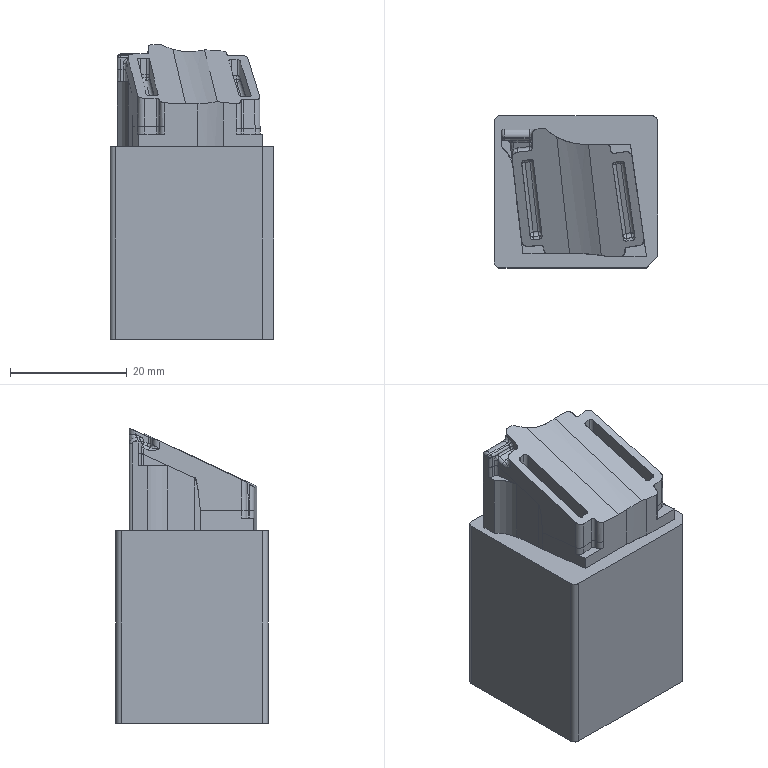NC program | NX | posted with a generic post | part box 28 x 26 x 50.455 mm
Whole program:
N10 G17 G21 G94 G90
(CAVITY_MILL_COPY_COPY , TOOL : MILL_2)
N12 T00 M6
N14 G54
N16 G17 G0 G90 X-14.496 Y12.325 S0 M3
N18 G43 Z10. H0
N20 Z-0.037
N22 G94 G1 Z-0.337 F250.
N24 X-13.997
N26 G3 X-10.997 Y9.325 R3.
N28 G1 X-9.23
N30 G2 X-8.224 Y10.006 R1.
N32 G1 Y9.972
N34 X-8.238 Y9.844
N36 G3 X-8.224 Y9.604 R0.772
N38 G1 X-8.223 Y9.02
N40 Y9.016
N42 X-8.193 Y8.822
N44 X-8.192 Y8.813
N46 X-8.193 Y8.451
N48 X-8.176 Y8.175
N50 Y8.168
N52 X-8.193 Y7.889
N54 Y7.705
N56 X-8.175 Y7.66
N58 X-8.223 Y7.653
N60 X-8.222 Y6.701
N62 X-8.235 Y6.699
N64 X-8.509 Y6.67
N66 X-8.781 Y6.639
N68 X-8.835 Y6.632
N70 X-8.877 Y6.628
N72 X-8.919 Y6.622
N74 X-8.93 Y6.621
N76 X-8.962 Y6.616
N78 X-9.071 Y6.605
N80 X-9.078 Y6.604
N82 X-9.335 Y6.574
N84 X-9.34 Y6.573
N86 X-9.475 Y6.558
N88 X-9.537 Y6.55
N90 X-9.569 Y6.546
N92 X-9.688 Y6.538
N94 X-9.815 Y6.524
N96 X-9.884 Y6.511
N98 X-10.081 Y6.481
N100 X-10.09 Y6.478
N102 G2 X-10.266 Y6.367 R1.
N104 G1 X-10.453 Y6.274
N106 X-10.499 Y6.228
N108 X-10.528 Y6.189
N110 X-10.552 Y6.155
N112 X-10.588 Y6.093
N114 X-10.592 Y6.085
N116 X-10.651 Y5.932
N118 X-10.661 Y5.89
N120 X-10.673 Y5.816
N122 Y5.536
N124 G2 X-12.665 Y5.416 R1.
N126 X-12.582 Y6.741 R3.632
N128 G1 X-12.559 Y6.816
N130 X-12.496 Y7.003
N132 G2 X-13.262 Y7.975 R1.
N134 G1 X-13.263 Y8.325
N136 G2 X-12.263 Y9.325 R1.
N138 G1 X-10.997
N140 Y9.075
N142 X-9.23
N144 G3 X-8.993 Y9.246 R0.25
N146 G2 X-8.491 Y9.728 R0.75
N148 G1 X-8.474 Y9.579
N150 X-8.473 Y8.993
N152 X-8.469 Y8.972
N154 X-8.442 Y8.799
N156 X-8.443 Y8.444
N158 X-8.427 Y8.171
N160 X-8.443 Y7.897
N162 Y7.772
N164 X-8.495 Y7.722
N166 X-8.473 Y7.653
N168 Y6.925
N170 X-8.536 Y6.918
N172 X-8.81 Y6.887
N174 X-8.865 Y6.88
N176 X-8.896 Y6.877
N178 X-8.906
N180 X-8.916 Y6.875
N182 X-8.948 Y6.871
N184 X-8.963 Y6.869
N186 X-9.001 Y6.863
N188 X-9.092 Y6.854
N190 X-9.102 Y6.853
N192 X-9.601 Y6.794
N194 X-9.703 Y6.788
N196 X-9.856 Y6.771
N198 X-9.869 Y6.768
N200 X-9.921 Y6.758
N202 X-10.136 Y6.725
N204 X-10.207 Y6.734
N206 X-10.245 Y6.674
N208 X-10.377 Y6.591
N210 X-10.564 Y6.498
N212 X-10.629 Y6.451
N214 X-10.688 Y6.393
N216 X-10.731 Y6.336
N218 X-10.763 Y6.29
N220 X-10.807 Y6.214
N222 X-10.821 Y6.188
N224 X-10.891 Y6.005
N226 X-10.906 Y5.937
N228 X-10.923 Y5.836
N230 Y5.536
N232 G2 X-12.417 Y5.446 R0.75
N234 X-12.322 Y6.736 R3.382
N236 G1 X-12.259 Y6.923
N238 G3 X-12.438 Y7.246 R0.25
N240 G2 X-13.012 Y7.975 R0.75
N242 G1 X-13.013 Y8.325
N244 G2 X-12.263 Y9.075 R0.75
N246 G1 X-10.997
N248 Y8.825
N250 X-9.23
N252 G3 X-8.756 Y9.166 R0.5
N254 G1 X-8.724 Y9.242
N256 X-8.723 Y8.965
N258 X-8.715 Y8.926
N260 X-8.692 Y8.78
N262 X-8.693 Y8.437
N264 X-8.677 Y8.172
N266 X-8.693 Y7.904
N268 Y7.824
N270 X-8.745 Y7.745
N272 X-8.723 Y7.652
N274 Y7.149
N276 X-8.839 Y7.135
N278 X-8.891 Y7.129
N280 X-8.918 Y7.126
N282 X-8.935 Y7.125
N284 X-8.953 Y7.122
N286 X-8.979 Y7.119
N288 X-8.997 Y7.117
N290 X-9.041 Y7.11
N292 X-9.113 Y7.104
N294 X-9.132 Y7.101
N296 X-9.631 Y7.042
N298 X-9.716 Y7.039
N300 X-9.898 Y7.017
N302 X-9.92 Y7.013
N304 X-9.963 Y7.004
N306 X-10.179 Y6.972
N308 G3 X-10.401 Y6.87 R0.5
N310 G1 X-10.489 Y6.815
N312 X-10.675 Y6.722
N314 X-10.806 Y6.629
N316 X-10.878 Y6.557
N318 X-10.933 Y6.482
N320 X-10.974 Y6.425
N322 X-11.026 Y6.335
N324 X-11.049 Y6.291
N326 X-11.131 Y6.077
N328 X-11.152 Y5.984
N330 X-11.173 Y5.856
N332 Y5.536
N334 G2 X-12.169 Y5.476 R0.5
N336 X-12.083 Y6.663 R3.132
N338 G1 X-12.022 Y6.843
N340 G3 X-12.379 Y7.489 R0.5
N342 G2 X-12.762 Y7.975 R0.5
N344 G1 X-12.763 Y8.325
N346 G2 X-12.263 Y8.825 R0.5
N348 G1 X-10.997
N350 Y8.575
N352 X-9.23
N354 G3 X-8.942 Y8.633 R0.75
N356 G1 X-8.943 Y8.43
N358 X-8.928 Y8.172
N360 X-8.943 Y7.912
N362 Y7.864
N364 G3 X-8.973 Y7.652 R0.75
N366 G1 Y7.372
N368 X-8.989 Y7.37
N370 X-9.01 Y7.367
N372 X-9.031 Y7.364
N374 X-9.08 Y7.357
N376 X-9.13 Y7.353
N378 X-9.162 Y7.349
N380 X-9.662 Y7.291
N382 X-9.726 Y7.289
N384 X-9.94 Y7.264
N386 X-9.97 Y7.258
N388 X-10.005 Y7.251
N390 X-10.221 Y7.218
N392 G3 X-10.557 Y7.065 R0.75
N394 G1 X-10.6 Y7.039
N396 X-10.786 Y6.946
N398 G3 X-10.982 Y6.806 R0.75
N400 G1 X-11.067 Y6.721
N402 X-11.136 Y6.629
N404 X-11.184 Y6.56
N406 X-11.245 Y6.455
N408 X-11.277 Y6.393
N410 X-11.371 Y6.15
N412 X-11.398 Y6.031
N414 X-11.423 Y5.876
N416 Y5.536
N418 G2 X-11.921 Y5.506 R0.25
N420 X-11.844 Y6.591 R2.882
N422 G1 X-11.786 Y6.763
N424 G3 X-12.321 Y7.732 R0.75
N426 G2 X-12.512 Y7.975 R0.25
N428 G1 X-12.513 Y8.325
N430 G2 X-12.263 Y8.575 R0.25
N432 G1 X-10.997
N434 X-10.996 Y8.325
N436 X-9.187 Y8.326
N438 X-9.178 Y8.172
N440 X-9.193 Y7.919
N442 Y7.897
N444 G3 X-9.223 Y7.652 R1.
N446 G1 Y7.594
N448 X-9.695 Y7.538
N450 X-9.7
N452 X-9.727 Y7.541
N454 X-9.982 Y7.511
N456 X-10.02 Y7.502
N458 X-10.046 Y7.498
N460 X-10.262 Y7.465
N462 G3 X-10.711 Y7.263 R1.
N464 G1 X-10.897 Y7.17
N466 G3 X-11.158 Y6.983 R1.
N468 G1 X-11.257 Y6.885
N470 X-11.339 Y6.775
N472 X-11.395 Y6.695
N474 X-11.464 Y6.576
N476 X-11.506 Y6.496
N478 X-11.611 Y6.223
N480 X-11.643 Y6.079
N482 X-11.673 Y5.896
N484 Y5.536
N486 G2 X-11.604 Y6.519 R2.632
N488 G1 X-11.549 Y6.683
N490 G3 X-12.262 Y7.975 R1.
N492 G1 X-12.263 Y8.325
N494 X-10.996
N496 Y8.075
N498 X-9.434 Y8.076
N500 X-9.443 Y7.926
N502 X-9.463 Y7.817
N504 X-9.702 Y7.789
N506 X-9.729 Y7.792
N508 X-10.024 Y7.758
N510 X-10.071 Y7.747
N512 X-10.088 Y7.744
N514 X-10.302 Y7.712
N516 G3 X-10.844 Y7.475 R1.25
N518 G1 X-11.008 Y7.394
N520 G3 X-11.266 Y7.224 R1.25
N522 X-11.853 Y8.075 R1.25
N524 G1 X-10.996
N526 Y7.825
N528 X-10.751 Y7.826
N530 G3 X-10.976 Y7.689 R1.5
N532 G1 X-11.119 Y7.618
N534 X-11.126 Y7.615
N536 G3 X-11.242 Y7.825 R1.5
N538 G1 X-10.996
N540 G3 X-9.497 Y9.326 R1.5
N542 G1 Z-0.037
N544 G0 Z0.3
N546 X-14.496 Y12.325
N548 Z-0.374
N550 G1 Z-0.674
N552 X-13.997
N554 G3 X-10.997 Y9.325 R3.
N556 G1 X-9.23
N558 G2 X-8.228 Y10.006 R1.
N560 G3 X-8.252 Y9.716 R1.75
N562 G1 Y9.152
N564 G3 X-8.192 Y8.769 R0.811
N566 G1 X-8.193 Y8.451
N568 X-8.176 Y8.175
N570 Y8.168
N572 X-8.193 Y7.889
N574 Y7.705
N576 X-8.175 Y7.66
N578 X-8.223 Y7.653
N580 X-8.222 Y6.701
N582 X-8.235 Y6.699
N584 X-8.509 Y6.67
N586 X-8.781 Y6.639
N588 X-8.835 Y6.632
N590 X-8.877 Y6.628
N592 X-8.919 Y6.622
N594 X-8.93 Y6.621
N596 X-8.962 Y6.616
N598 X-9.071 Y6.605
N600 X-9.078 Y6.604
N602 X-9.335 Y6.574
N604 X-9.34 Y6.573
N606 X-9.475 Y6.558
N608 X-9.537 Y6.55
N610 X-9.569 Y6.546
N612 X-9.688 Y6.538
N614 X-9.815 Y6.524
N616 X-9.884 Y6.511
N618 X-10.081 Y6.481
N620 X-10.09 Y6.478
N622 G2 X-10.266 Y6.367 R1.
N624 G1 X-10.453 Y6.274
N626 X-10.499 Y6.228
N628 X-10.528 Y6.189
N630 X-10.552 Y6.155
N632 X-10.588 Y6.093
N634 X-10.592 Y6.085
N636 X-10.651 Y5.932
N638 X-10.661 Y5.89
N640 X-10.673 Y5.816
N642 Y5.536
N644 G2 X-12.665 Y5.416 R1.
N646 X-12.582 Y6.741 R3.632
N648 G1 X-12.559 Y6.816
N650 X-12.496 Y7.003
N652 G2 X-13.262 Y7.975 R1.
N654 G1 X-13.263 Y8.325
N656 G2 X-12.263 Y9.325 R1.
N658 G1 X-10.997
N660 Y9.075
N662 X-9.23
N664 G3 X-8.993 Y9.246 R0.25
N666 G2 X-8.502 Y9.724 R0.75
N668 G1 Y9.715
N670 Y9.162
N672 G3 X-8.442 Y8.722 R1.061
N674 G1 X-8.443 Y8.444
N676 X-8.427 Y8.171
N678 X-8.443 Y7.897
N680 Y7.772
N682 X-8.495 Y7.722
N684 X-8.473 Y7.653
N686 Y6.925
N688 X-8.536 Y6.918
N690 X-8.81 Y6.887
N692 X-8.865 Y6.88
N694 X-8.896 Y6.877
N696 X-8.906
N698 X-8.916 Y6.875
N700 X-9.001 Y6.863
N702 X-9.092 Y6.854
N704 X-9.102 Y6.853
N706 X-9.108 Y6.852
N708 X-9.364 Y6.822
N710 X-9.368 Y6.821
N712 X-9.504 Y6.806
N714 X-9.568 Y6.798
N716 X-9.703 Y6.788
N718 X-9.856 Y6.771
N720 X-9.869 Y6.768
N722 X-9.921 Y6.758
N724 X-10.136 Y6.725
N726 X-10.207 Y6.734
N728 X-10.245 Y6.674
N730 X-10.377 Y6.591
N732 X-10.564 Y6.498
N734 X-10.629 Y6.451
N736 X-10.688 Y6.393
N738 X-10.731 Y6.336
N740 X-10.763 Y6.29
N742 X-10.807 Y6.214
N744 X-10.821 Y6.188
N746 X-10.891 Y6.005
N748 X-10.906 Y5.937
N750 X-10.923 Y5.836
N752 Y5.536
N754 G2 X-12.417 Y5.446 R0.75
N756 X-12.322 Y6.736 R3.382
N758 G1 X-12.259 Y6.923
N760 G3 X-12.438 Y7.246 R0.25
N762 G2 X-13.012 Y7.975 R0.75
N764 G1 X-13.013 Y8.325
N766 G2 X-12.263 Y9.075 R0.75
N768 G1 X-10.997
N770 Y8.825
N772 X-9.23
N774 G3 X-8.756 Y9.166 R0.5
N776 G1 X-8.752 Y9.178
N778 G3 X-8.692 Y8.681 R1.311
N780 G1 X-8.693 Y8.437
N782 X-8.677 Y8.172
N784 X-8.693 Y7.904
N786 Y7.824
N788 X-8.745 Y7.745
N790 X-8.723 Y7.652
N792 Y7.149
N794 X-8.839 Y7.135
N796 X-8.891 Y7.129
N798 X-8.918 Y7.126
N800 X-8.935 Y7.125
N802 X-8.954 Y7.122
N804 X-9.039 Y7.11
N806 X-9.113 Y7.104
N808 X-9.133 Y7.101
N810 X-9.137 Y7.1
N812 X-9.393 Y7.07
N814 X-9.396
N816 X-9.533 Y7.055
N818 X-9.603 Y7.046
N820 X-9.715 Y7.039
N822 X-9.898 Y7.017
N824 X-9.92 Y7.013
N826 X-9.963 Y7.004
N828 X-10.179 Y6.972
N830 G3 X-10.401 Y6.87 R0.5
N832 G1 X-10.489 Y6.815
N834 X-10.675 Y6.722
N836 X-10.806 Y6.629
N838 X-10.878 Y6.557
N840 X-10.933 Y6.482
N842 X-10.974 Y6.425
N844 X-11.026 Y6.335
N846 X-11.049 Y6.291
N848 X-11.131 Y6.077
N850 X-11.152 Y5.984
N852 X-11.173 Y5.856
N854 Y5.536
N856 G2 X-12.169 Y5.476 R0.5
N858 X-12.083 Y6.663 R3.132
N860 G1 X-12.022 Y6.843
N862 G3 X-12.379 Y7.489 R0.5
N864 G2 X-12.762 Y7.975 R0.5
N866 G1 X-12.763 Y8.325
N868 G2 X-12.263 Y8.825 R0.5
N870 G1 X-10.997
N872 Y8.575
N874 X-9.23
N876 G3 X-8.942 Y8.633 R0.75
N878 G1 X-8.943 Y8.43
N880 X-8.928 Y8.172
N882 X-8.943 Y7.912
N884 Y7.864
N886 G3 X-8.973 Y7.652 R0.75
N888 G1 Y7.372
N890 X-8.991 Y7.37
N892 X-9.077 Y7.357
N894 X-9.13 Y7.353
N896 X-9.163 Y7.349
N898 X-9.167
N900 X-9.422 Y7.319
N902 X-9.425 Y7.318
N904 X-9.562 Y7.303
N906 X-9.641 Y7.293
N908 X-9.724 Y7.289
N910 X-9.94 Y7.264
N912 X-9.97 Y7.258
N914 X-10.005 Y7.251
N916 X-10.221 Y7.218
N918 G3 X-10.557 Y7.065 R0.75
N920 G1 X-10.6 Y7.039
N922 X-10.786 Y6.946
N924 G3 X-10.982 Y6.806 R0.75
N926 G1 X-11.067 Y6.721
N928 X-11.136 Y6.629
N930 X-11.184 Y6.56
N932 X-11.245 Y6.455
N934 X-11.277 Y6.393
N936 X-11.371 Y6.15
N938 X-11.398 Y6.031
N940 X-11.423 Y5.876
N942 Y5.536
N944 G2 X-11.921 Y5.506 R0.25
N946 X-11.844 Y6.591 R2.882
N948 G1 X-11.786 Y6.763
N950 G3 X-12.321 Y7.732 R0.75
N952 G2 X-12.512 Y7.975 R0.25
N954 G1 X-12.513 Y8.325
N956 G2 X-12.263 Y8.575 R0.25
N958 G1 X-10.997
N960 X-10.996 Y8.325
N962 X-9.187 Y8.326
N964 X-9.178 Y8.172
N966 X-9.193 Y7.919
N968 Y7.897
N970 G3 X-9.223 Y7.652 R1.
N972 G1 Y7.594
N974 X-9.451 Y7.567
N976 X-9.453
N978 X-9.591 Y7.551
N980 X-9.683 Y7.54
N982 X-9.694 Y7.537
N984 X-9.724 Y7.541
N986 X-9.982 Y7.511
N988 X-10.02 Y7.502
N990 X-10.046 Y7.498
N992 X-10.262 Y7.465
N994 G3 X-10.711 Y7.263 R1.
N996 G1 X-10.897 Y7.17
N998 G3 X-11.158 Y6.983 R1.
N1000 G1 X-11.257 Y6.885
N1002 X-11.339 Y6.775
N1004 X-11.395 Y6.695
N1006 X-11.464 Y6.576
N1008 X-11.506 Y6.496
N1010 X-11.611 Y6.223
N1012 X-11.643 Y6.079
N1014 X-11.673 Y5.896
N1016 Y5.536
N1018 G2 X-11.604 Y6.519 R2.632
N1020 G1 X-11.549 Y6.683
N1022 G3 X-12.262 Y7.975 R1.
N1024 G1 X-12.263 Y8.325
N1026 X-10.996
N1028 Y8.075
N1030 X-9.434 Y8.076
N1032 X-9.443 Y7.926
N1034 X-9.463 Y7.817
N1036 X-9.48 Y7.815
N1038 X-9.481
N1040 X-9.62 Y7.799
N1042 X-9.699 Y7.79
N1044 X-9.723 Y7.793
N1046 X-10.024 Y7.758
N1048 X-10.071 Y7.747
N1050 X-10.088 Y7.744
N1052 X-10.302 Y7.712
N1054 G3 X-10.844 Y7.475 R1.25
N1056 G1 X-11.008 Y7.394
N1058 G3 X-11.266 Y7.224 R1.25
N1060 X-11.853 Y8.075 R1.25
N1062 G1 X-10.996
N1064 Y7.825
N1066 X-10.751 Y7.826
N1068 G3 X-10.976 Y7.689 R1.5
N1070 G1 X-11.119 Y7.618
N1072 X-11.126 Y7.615
N1074 G3 X-11.242 Y7.825 R1.5
N1076 G1 X-10.996
N1078 G3 X-9.497 Y9.326 R1.5
N1080 G1 Z-0.374
N1082 G0 Z0.3
N1084 X-14.496 Y12.325
N1086 Z-0.71
N1088 G1 Z-1.01
N1090 X-13.997
N1092 G3 X-10.997 Y9.325 R3.
N1094 G1 X-9.23
N1096 G2 X-8.234 Y10.006 R1.
N1098 G3 X-8.254 Y9.612 R1.746
N1100 G1 X-8.253 Y8.425
N1102 G3 X-8.185 Y8.024 R0.811
N1104 G1 X-8.193 Y7.889
N1106 Y7.705
N1108 X-8.175 Y7.66
N1110 X-8.223 Y7.653
N1112 X-8.222 Y6.701
N1114 X-8.235 Y6.699
N1116 X-8.509 Y6.67
N1118 X-8.781 Y6.639
N1120 X-8.835 Y6.632
N1122 X-8.877 Y6.628
N1124 X-8.919 Y6.622
N1126 X-8.93 Y6.621
N1128 X-8.962 Y6.616
N1130 X-9.071 Y6.605
N1132 X-9.078 Y6.604
N1134 X-9.335 Y6.574
N1136 X-9.34 Y6.573
N1138 X-9.475 Y6.558
N1140 X-9.537 Y6.55
N1142 X-9.569 Y6.546
N1144 X-9.688 Y6.538
N1146 X-9.815 Y6.524
N1148 X-9.884 Y6.511
N1150 X-10.081 Y6.481
N1152 X-10.09 Y6.478
N1154 G2 X-10.266 Y6.367 R1.
N1156 G1 X-10.453 Y6.274
N1158 X-10.499 Y6.228
N1160 X-10.528 Y6.189
N1162 X-10.552 Y6.155
N1164 X-10.588 Y6.093
N1166 X-10.592 Y6.085
N1168 X-10.651 Y5.932
N1170 X-10.661 Y5.89
N1172 X-10.673 Y5.816
N1174 Y5.536
N1176 G2 X-12.665 Y5.416 R1.
N1178 X-12.582 Y6.741 R3.632
N1180 G1 X-12.559 Y6.816
N1182 X-12.496 Y7.003
N1184 G2 X-13.262 Y7.975 R1.
N1186 G1 X-13.263 Y8.325
N1188 G2 X-12.263 Y9.325 R1.
N1190 G1 X-10.997
N1192 Y9.075
N1194 X-9.23
N1196 G3 X-8.993 Y9.246 R0.25
N1198 G2 X-8.507 Y9.723 R0.75
N1200 G1 X-8.504 Y9.604
N1202 X-8.503 Y8.435
N1204 G3 X-8.438 Y7.982 R1.061
N1206 G1 X-8.443 Y7.897
N1208 Y7.772
N1210 X-8.495 Y7.722
N1212 X-8.473 Y7.653
N1214 Y6.925
N1216 X-8.536 Y6.918
N1218 X-8.81 Y6.887
N1220 X-8.865 Y6.88
N1222 X-8.896 Y6.877
N1224 X-8.906
N1226 X-8.916 Y6.875
N1228 X-9.001 Y6.863
N1230 X-9.092 Y6.854
N1232 X-9.102 Y6.853
N1234 X-9.108 Y6.852
N1236 X-9.364 Y6.822
N1238 X-9.601 Y6.794
N1240 X-9.703 Y6.788
N1242 X-9.856 Y6.771
N1244 X-9.869 Y6.768
N1246 X-9.921 Y6.758
N1248 X-10.136 Y6.725
N1250 X-10.207 Y6.734
N1252 X-10.245 Y6.674
N1254 X-10.377 Y6.591
N1256 X-10.564 Y6.498
N1258 X-10.629 Y6.451
N1260 X-10.688 Y6.393
N1262 X-10.731 Y6.336
N1264 X-10.763 Y6.29
N1266 X-10.807 Y6.214
N1268 X-10.821 Y6.188
N1270 X-10.891 Y6.005
N1272 X-10.906 Y5.937
N1274 X-10.923 Y5.836
N1276 Y5.536
N1278 G2 X-12.417 Y5.446 R0.75
N1280 X-12.322 Y6.736 R3.382
N1282 G1 X-12.259 Y6.923
N1284 G3 X-12.438 Y7.246 R0.25
N1286 G2 X-13.012 Y7.975 R0.75
N1288 G1 X-13.013 Y8.325
N1290 G2 X-12.263 Y9.075 R0.75
N1292 G1 X-10.997
N1294 Y8.825
N1296 X-9.23
N1298 G3 X-8.756 Y9.166 R0.5
N1300 G1 X-8.753 Y9.173
N1302 Y8.444
N1304 G3 X-8.691 Y7.947 R1.311
N1306 G1 X-8.693 Y7.904
N1308 Y7.824
N1310 X-8.745 Y7.745
N1312 X-8.723 Y7.652
N1314 Y7.149
N1316 X-8.839 Y7.135
N1318 X-8.891 Y7.129
N1320 X-8.918 Y7.126
N1322 X-8.935 Y7.125
N1324 X-8.954 Y7.122
N1326 X-9.039 Y7.11
N1328 X-9.113 Y7.104
N1330 X-9.133 Y7.101
N1332 X-9.137 Y7.1
N1334 X-9.393 Y7.07
N1336 X-9.631 Y7.042
N1338 X-9.716 Y7.039
N1340 X-9.898 Y7.017
N1342 X-9.92 Y7.013
N1344 X-9.963 Y7.004
N1346 X-10.179 Y6.972
N1348 G3 X-10.401 Y6.87 R0.5
N1350 G1 X-10.489 Y6.815
N1352 X-10.675 Y6.722
N1354 X-10.806 Y6.629
N1356 X-10.878 Y6.557
N1358 X-10.933 Y6.482
N1360 X-10.974 Y6.425
N1362 X-11.026 Y6.335
N1364 X-11.049 Y6.291
N1366 X-11.131 Y6.077
N1368 X-11.152 Y5.984
N1370 X-11.173 Y5.856
N1372 Y5.536
N1374 G2 X-12.169 Y5.476 R0.5
N1376 X-12.083 Y6.663 R3.132
N1378 G1 X-12.022 Y6.843
N1380 G3 X-12.379 Y7.489 R0.5
N1382 G2 X-12.762 Y7.975 R0.5
N1384 G1 X-12.763 Y8.325
N1386 G2 X-12.263 Y8.825 R0.5
N1388 G1 X-10.997
N1390 Y8.575
N1392 X-9.23
N1394 G3 X-9.003 Y8.611 R0.75
N1396 G1 Y8.452
N1398 G3 X-8.943 Y7.912 R1.561
N1400 G1 Y7.864
N1402 G3 X-8.973 Y7.652 R0.75
N1404 G1 Y7.372
N1406 X-8.991 Y7.37
N1408 X-9.077 Y7.357
N1410 X-9.13 Y7.353
N1412 X-9.163 Y7.349
N1414 X-9.167
N1416 X-9.423 Y7.319
N1418 X-9.662 Y7.291
N1420 X-9.726 Y7.289
N1422 X-9.94 Y7.264
N1424 X-9.97 Y7.258
N1426 X-10.005 Y7.251
N1428 X-10.221 Y7.218
N1430 G3 X-10.557 Y7.065 R0.75
N1432 G1 X-10.6 Y7.039
N1434 X-10.786 Y6.946
N1436 G3 X-10.982 Y6.806 R0.75
N1438 G1 X-11.067 Y6.721
N1440 X-11.136 Y6.629
N1442 X-11.184 Y6.56
N1444 X-11.245 Y6.455
N1446 X-11.277 Y6.393
N1448 X-11.371 Y6.15
N1450 X-11.398 Y6.031
N1452 X-11.423 Y5.876
N1454 Y5.536
N1456 G2 X-11.921 Y5.506 R0.25
N1458 X-11.844 Y6.591 R2.882
N1460 G1 X-11.786 Y6.763
N1462 G3 X-12.321 Y7.732 R0.75
N1464 G2 X-12.512 Y7.975 R0.25
N1466 G1 X-12.513 Y8.325
N1468 G2 X-12.263 Y8.575 R0.25
N1470 G1 X-10.997
N1472 X-10.996 Y8.325
N1474 X-9.256
N1476 G3 X-9.196 Y7.886 R1.811
N1478 X-9.223 Y7.652 R1.
N1480 G1 Y7.594
N1482 X-9.452 Y7.567
N1484 X-9.695 Y7.538
N1486 X-9.7
N1488 X-9.727 Y7.541
N1490 X-9.982 Y7.511
N1492 X-10.02 Y7.502
N1494 X-10.046 Y7.498
N1496 X-10.262 Y7.465
N1498 G3 X-10.711 Y7.263 R1.
N1500 G1 X-10.897 Y7.17
N1502 G3 X-11.158 Y6.983 R1.
N1504 G1 X-11.257 Y6.885
N1506 X-11.339 Y6.775
N1508 X-11.395 Y6.695
N1510 X-11.464 Y6.576
N1512 X-11.506 Y6.496
N1514 X-11.611 Y6.223
N1516 X-11.643 Y6.079
N1518 X-11.673 Y5.896
N1520 Y5.536
N1522 G2 X-11.604 Y6.519 R2.632
N1524 G1 X-11.549 Y6.683
N1526 G3 X-12.262 Y7.975 R1.
N1528 G1 X-12.263 Y8.325
N1530 X-10.996
N1532 Y8.075
N1534 X-9.488
N1536 X-9.452 Y7.882
N1538 X-9.463 Y7.817
N1540 X-9.481 Y7.815
N1542 X-9.702 Y7.789
N1544 X-9.728 Y7.792
N1546 X-10.024 Y7.758
N1548 X-10.071 Y7.747
N1550 X-10.088 Y7.744
N1552 X-10.302 Y7.712
N1554 G3 X-10.844 Y7.475 R1.25
N1556 G1 X-11.008 Y7.394
N1558 G3 X-11.266 Y7.224 R1.25
N1560 X-11.853 Y8.075 R1.25
N1562 G1 X-10.996
N1564 Y7.825
N1566 X-10.752
N1568 G3 X-10.976 Y7.689 R1.5
N1570 G1 X-11.119 Y7.618
N1572 X-11.126 Y7.615
N1574 G3 X-11.241 Y7.825 R1.5
N1576 G1 X-10.996
N1578 G3 X-9.497 Y9.325 R1.5
N1580 G1 Z-0.71
N1582 G0 Z0.3
N1584 X-14.496 Y12.325
N1586 Z-1.047
N1588 G1 Z-1.347
N1590 X-13.997
N1592 G3 X-10.997 Y9.325 R3.
N1594 G1 X-9.23
N1596 G2 X-8.344 Y10.005 R1.
N1598 G3 X-8.264 Y9.007 R1.821
N1600 G1 X-8.255 Y8.898
N1602 X-8.253 Y7.698
N1604 G3 X-8.223 Y7.397 R0.811
N1606 G1 X-8.222 Y6.701
N1608 X-8.235 Y6.699
N1610 X-8.509 Y6.67
N1612 X-8.781 Y6.639
N1614 X-8.835 Y6.632
N1616 X-8.877 Y6.628
N1618 X-8.919 Y6.622
N1620 X-8.93 Y6.621
N1622 X-8.962 Y6.616
N1624 X-9.071 Y6.605
N1626 X-9.078 Y6.604
N1628 X-9.335 Y6.574
N1630 X-9.34 Y6.573
N1632 X-9.475 Y6.558
N1634 X-9.537 Y6.55
N1636 X-9.569 Y6.546
N1638 X-9.688 Y6.538
N1640 X-9.815 Y6.524
N1642 X-9.884 Y6.511
N1644 X-10.081 Y6.481
N1646 X-10.09 Y6.478
N1648 G2 X-10.266 Y6.367 R1.
N1650 G1 X-10.453 Y6.274
N1652 X-10.499 Y6.228
N1654 X-10.528 Y6.189
N1656 X-10.552 Y6.155
N1658 X-10.588 Y6.093
N1660 X-10.592 Y6.085
N1662 X-10.651 Y5.932
N1664 X-10.661 Y5.89
N1666 X-10.673 Y5.816
N1668 Y5.536
N1670 G2 X-12.665 Y5.416 R1.
N1672 X-12.582 Y6.741 R3.632
N1674 G1 X-12.559 Y6.816
N1676 X-12.496 Y7.003
N1678 G2 X-13.262 Y7.975 R1.
N1680 G1 X-13.263 Y8.325
N1682 G2 X-12.263 Y9.325 R1.
N1684 G1 X-10.997
N1686 Y9.075
N1688 X-9.23
N1690 G3 X-8.993 Y9.246 R0.25
N1692 G2 X-8.63 Y9.672 R0.75
N1694 G3 X-8.511 Y8.953 R2.071
N1696 G1 X-8.505 Y8.887
N1698 X-8.504 Y7.708
N1700 G3 X-8.473 Y7.363 R1.061
N1702 G1 Y6.925
N1704 X-8.536 Y6.918
N1706 X-8.81 Y6.887
N1708 X-8.865 Y6.88
N1710 X-8.896 Y6.877
N1712 X-8.906
N1714 X-8.916 Y6.875
N1716 X-8.948 Y6.871
N1718 X-8.963 Y6.869
N1720 X-9.001 Y6.863
N1722 X-9.092 Y6.854
N1724 X-9.102 Y6.853
N1726 X-9.108 Y6.852
N1728 X-9.364 Y6.822
N1730 X-9.601 Y6.794
N1732 X-9.703 Y6.788
N1734 X-9.856 Y6.771
N1736 X-9.869 Y6.768
N1738 X-9.921 Y6.758
N1740 X-10.136 Y6.725
N1742 X-10.207 Y6.734
N1744 X-10.245 Y6.674
N1746 X-10.377 Y6.591
N1748 X-10.564 Y6.498
N1750 X-10.629 Y6.451
N1752 X-10.688 Y6.393
N1754 X-10.731 Y6.336
N1756 X-10.763 Y6.29
N1758 X-10.807 Y6.214
N1760 X-10.821 Y6.188
N1762 X-10.891 Y6.005
N1764 X-10.906 Y5.937
N1766 X-10.923 Y5.836
N1768 Y5.536
N1770 G2 X-12.417 Y5.446 R0.75
N1772 X-12.322 Y6.736 R3.382
N1774 G1 X-12.259 Y6.923
N1776 G3 X-12.438 Y7.246 R0.25
N1778 G2 X-13.012 Y7.975 R0.75
N1780 G1 X-13.013 Y8.325
N1782 G2 X-12.263 Y9.075 R0.75
N1784 G1 X-10.997
N1786 Y8.825
N1788 X-9.23
N1790 G3 X-8.805 Y9.061 R0.5
N1792 G1 X-8.757 Y8.9
N1794 X-8.755 Y8.876
N1796 X-8.754 Y7.717
N1798 G3 X-8.723 Y7.333 R1.311
N1800 G1 Y7.149
N1802 X-8.839 Y7.135
N1804 X-8.891 Y7.129
N1806 X-8.918 Y7.126
N1808 X-8.935 Y7.125
N1810 X-8.953 Y7.122
N1812 X-8.979 Y7.119
N1814 X-8.997 Y7.117
N1816 X-9.041 Y7.11
N1818 X-9.113 Y7.104
N1820 X-9.133 Y7.101
N1822 X-9.137 Y7.1
N1824 X-9.393 Y7.07
N1826 X-9.631 Y7.042
N1828 X-9.716 Y7.039
N1830 X-9.898 Y7.017
N1832 X-9.92 Y7.013
N1834 X-9.963 Y7.004
N1836 X-10.179 Y6.972
N1838 G3 X-10.401 Y6.87 R0.5
N1840 G1 X-10.489 Y6.815
N1842 X-10.675 Y6.722
N1844 X-10.806 Y6.629
N1846 X-10.878 Y6.557
N1848 X-10.933 Y6.482
N1850 X-10.974 Y6.425
N1852 X-11.026 Y6.335
N1854 X-11.049 Y6.291
N1856 X-11.131 Y6.077
N1858 X-11.152 Y5.984
N1860 X-11.173 Y5.856
N1862 Y5.536
N1864 G2 X-12.169 Y5.476 R0.5
N1866 X-12.083 Y6.663 R3.132
N1868 G1 X-12.022 Y6.843
N1870 G3 X-12.379 Y7.489 R0.5
N1872 G2 X-12.762 Y7.975 R0.5
N1874 G1 X-12.763 Y8.325
N1876 G2 X-12.263 Y8.825 R0.5
N1878 G1 X-10.997
N1880 Y8.575
N1882 X-9.23
N1884 G3 X-9.005 Y8.61 R0.75
N1886 G1 X-9.004 Y7.725
N1888 G3 X-8.985 Y7.37 R1.561
N1890 G1 X-8.989
N1892 X-9.01 Y7.367
N1894 X-9.031 Y7.364
N1896 X-9.08 Y7.357
N1898 X-9.13 Y7.353
N1900 X-9.163 Y7.349
N1902 X-9.167
N1904 X-9.423 Y7.319
N1906 X-9.662 Y7.291
N1908 X-9.726 Y7.289
N1910 X-9.94 Y7.264
N1912 X-9.97 Y7.258
N1914 X-10.005 Y7.251
N1916 X-10.221 Y7.218
N1918 G3 X-10.557 Y7.065 R0.75
N1920 G1 X-10.6 Y7.039
N1922 X-10.786 Y6.946
N1924 G3 X-10.982 Y6.806 R0.75
N1926 G1 X-11.067 Y6.721
N1928 X-11.136 Y6.629
N1930 X-11.184 Y6.56
N1932 X-11.245 Y6.455
N1934 X-11.277 Y6.393
N1936 X-11.371 Y6.15
N1938 X-11.398 Y6.031
N1940 X-11.423 Y5.876
N1942 Y5.536
N1944 G2 X-11.921 Y5.506 R0.25
N1946 X-11.844 Y6.591 R2.882
N1948 G1 X-11.786 Y6.763
N1950 G3 X-12.321 Y7.732 R0.75
N1952 G2 X-12.512 Y7.975 R0.25
N1954 G1 X-12.513 Y8.325
N1956 G2 X-12.263 Y8.575 R0.25
N1958 G1 X-10.997
N1960 X-10.996 Y8.325
N1962 X-9.254
N1964 Y7.732
N1966 X-9.256 Y7.59
N1968 X-9.452 Y7.567
N1970 X-9.695 Y7.538
N1972 X-9.7
N1974 X-9.727 Y7.541
N1976 X-9.982 Y7.511
N1978 X-10.02 Y7.502
N1980 X-10.046 Y7.498
N1982 X-10.262 Y7.465
N1984 G3 X-10.711 Y7.263 R1.
N1986 G1 X-10.897 Y7.17
N1988 G3 X-11.158 Y6.983 R1.
N1990 G1 X-11.257 Y6.885
N1992 X-11.339 Y6.775
N1994 X-11.395 Y6.695
N1996 X-11.464 Y6.576
N1998 X-11.506 Y6.496
N2000 X-11.611 Y6.223
N2002 X-11.643 Y6.079
N2004 X-11.673 Y5.896
N2006 Y5.536
N2008 G2 X-11.604 Y6.519 R2.632
N2010 G1 X-11.549 Y6.683
N2012 G3 X-12.262 Y7.975 R1.
N2014 G1 X-12.263 Y8.325
N2016 X-10.996
N2018 Y8.075
N2020 X-9.504
N2022 Y7.812
N2024 X-9.702 Y7.789
N2026 X-9.728 Y7.792
N2028 X-10.024 Y7.758
N2030 X-10.071 Y7.747
N2032 X-10.088 Y7.744
N2034 X-10.302 Y7.712
N2036 G3 X-10.844 Y7.475 R1.25
N2038 G1 X-11.008 Y7.394
N2040 G3 X-11.266 Y7.224 R1.25
N2042 X-11.853 Y8.075 R1.25
N2044 G1 X-10.996
N2046 Y7.825
N2048 X-10.752
N2050 G3 X-10.976 Y7.689 R1.5
N2052 G1 X-11.119 Y7.618
N2054 X-11.126 Y7.615
N2056 G3 X-11.241 Y7.825 R1.5
N2058 G1 X-10.996
N2060 G3 X-9.497 Y9.325 R1.5
N2062 G1 Z-1.047
N2064 G0 Z0.3
N2066 X-14.496 Y8.614
N2068 Z-1.384
N2070 G1 Z-1.684
N2072 G3 X-12.496 Y7.003 R3.
N2074 G2 X-13.262 Y7.975 R1.
N2076 G1 X-13.263 Y8.325
N2078 X-13.257 Y8.429
N2080 X-12.731 Y8.081
N2082 X-12.322 Y8.082
N2084 X-12.323 Y8.325
N2086 X-12.326 Y8.389
N2088 X-12.263 Y8.385
N2090 X-8.342
N2092 X-8.343 Y8.431
N2094 X-8.346 Y8.482
N2096 X-8.268
N2098 X-8.256 Y8.419
N2100 X-8.255 Y7.706
N2102 X-10.116 Y7.49
N2104 X-10.422 Y7.423
N2106 X-10.532 Y7.389
N2108 X-10.541 Y7.383
N2110 X-10.562 Y7.377
N2112 X-10.704 Y7.311
N2114 G3 X-11.267 Y6.775 R1.186
N2116 G1 X-11.274 Y6.761
N2118 X-11.29 Y6.74
N2120 X-11.345 Y6.662
N2122 X-11.412 Y6.547
N2124 X-11.451 Y6.471
N2126 X-11.545 Y6.228
N2128 X-11.555 Y6.2
N2130 X-11.584 Y6.067
N2132 X-11.613 Y5.891
N2134 Y5.536
N2136 X-11.593 Y5.495
N2138 X-11.638 Y5.487
N2140 X-11.528 Y4.547
N2142 G2 X-12.665 Y5.416 R1.
N2144 X-12.582 Y6.741 R3.632
N2146 G1 X-12.559 Y6.816
N2148 X-12.496 Y7.003
N2150 X-12.259 Y6.923
N2152 G3 X-12.438 Y7.246 R0.25
N2154 G2 X-13.012 Y7.968 R0.75
N2156 G1 X-12.869 Y7.873
N2158 X-12.811 Y7.813
N2160 X-12.73 Y7.831
N2162 X-12.322 Y7.832
N2164 G3 X-12.072 Y8.082 R0.25
N2166 G1 Y8.135
N2168 X-8.506
N2170 Y7.929
N2172 X-10.157 Y7.737
N2174 X-10.475 Y7.667
N2176 X-10.494 Y7.662
N2178 X-10.605 Y7.628
N2180 X-10.642 Y7.614
N2182 X-10.668 Y7.603
N2184 X-10.808 Y7.538
N2186 G3 X-11.486 Y6.895 R1.436
N2188 G1 X-11.493 Y6.886
N2190 X-11.555 Y6.797
N2192 X-11.631 Y6.667
N2194 X-11.679 Y6.574
N2196 X-11.779 Y6.315
N2198 X-11.795 Y6.27
N2200 X-11.83 Y6.115
N2202 X-11.863 Y5.911
N2204 Y5.597
N2206 X-11.914 Y5.534
N2208 X-11.886 Y5.458
N2210 X-11.809 Y4.799
N2212 G2 X-12.417 Y5.446 R0.75
N2214 X-12.322 Y6.736 R3.382
N2216 G1 X-12.259 Y6.923
N2218 X-12.022 Y6.843
N2220 G3 X-12.379 Y7.489 R0.5
N2222 G2 X-12.571 Y7.582 R0.5
N2224 G1 X-12.321
N2226 G3 X-11.863 Y7.885 R0.5
N2228 G1 X-10.619
N2230 X-10.678 Y7.867
N2232 X-10.742 Y7.843
N2234 X-10.761 Y7.835
N2236 X-10.774 Y7.83
N2238 X-10.913 Y7.765
N2240 G3 X-11.699 Y7.028 R1.686
N2242 G1 X-11.766 Y6.932
N2244 X-11.85 Y6.788
N2246 X-11.908 Y6.677
N2248 X-12.014 Y6.402
N2250 X-12.036 Y6.34
N2252 X-12.076 Y6.162
N2254 X-12.113 Y5.931
N2256 Y5.645
N2258 G3 X-12.135 Y5.429 R0.5
N2260 G1 X-12.121 Y5.316
N2262 X-12.169 Y5.476
N2264 G2 X-12.083 Y6.663 R3.132
N2266 G1 X-12.022 Y6.843
N2268 X-11.815 Y7.318
N2270 X-11.902 Y7.461
N2272 G3 X-11.721 Y7.635 R0.75
N2274 G1 X-11.546
N2276 G3 X-11.815 Y7.318 R1.936
N2278 X-11.016 Y3.151 R3.
N2280 G1 Z-1.384
N2282 G0 Z0.3
N2284 X-14.496 Y8.614
N2286 Z-1.721
N2288 G1 Z-2.021
N2290 G3 X-12.496 Y7.003 R3.
N2292 G2 X-13.262 Y7.975 R1.
N2294 G1 X-13.263 Y8.325
N2296 X-13.257 Y8.429
N2298 X-12.731 Y8.081
N2300 X-12.526 Y8.082
N2302 G3 X-12.262 Y8.053 R1.174
N2304 G1 X-8.342 Y8.061
N2306 X-8.257 Y8.068
N2308 Y7.708
N2310 X-10.119 Y7.492
N2312 G3 X-11.607 Y6.233 R1.714
N2314 G1 X-11.639 Y6.105
N2316 X-11.665 Y5.934
N2318 G3 X-11.623 Y5.502 R0.829
N2320 G1 X-11.638 Y5.487
N2322 X-11.528 Y4.547
N2324 G2 X-12.665 Y5.416 R1.
N2326 X-12.582 Y6.741 R3.632
N2328 G1 X-12.559 Y6.816
N2330 X-12.496 Y7.003
N2332 X-12.268 Y7.105
N2334 G3 X-12.438 Y7.246 R0.25
N2336 G2 X-13.012 Y7.968 R0.75
N2338 G1 X-12.869 Y7.873
N2340 X-12.811 Y7.813
N2342 X-12.73 Y7.831
N2344 X-12.553 Y7.832
N2346 G3 X-12.262 Y7.803 R1.424
N2348 G1 X-9.559 Y7.808
N2350 X-10.145 Y7.74
N2352 G3 X-11.849 Y6.296 R1.964
N2354 G1 X-11.884 Y6.155
N2356 X-11.912 Y5.973
N2358 G3 X-11.887 Y5.507 R1.079
N2360 G1 X-11.886 Y5.458
N2362 X-11.809 Y4.799
N2364 G2 X-12.417 Y5.446 R0.75
N2366 X-12.322 Y6.736 R3.382
N2368 G1 X-12.259 Y6.923
N2370 X-12.216 Y7.016
N2372 X-12.268 Y7.105
N2374 X-12.039 Y7.206
N2376 G3 X-12.379 Y7.489 R0.5
N2378 G2 X-12.569 Y7.58 R0.5
N2380 G3 X-12.261 Y7.553 R1.674
N2382 G1 X-11.284 Y7.555
N2384 G3 X-12.091 Y6.359 R2.214
N2386 G1 X-12.129 Y6.204
N2388 X-12.158 Y6.013
N2390 G3 X-12.138 Y5.477 R1.329
N2392 G1 X-12.135 Y5.429
N2394 X-12.121 Y5.316
N2396 X-12.169 Y5.476
N2398 G2 X-12.083 Y6.663 R3.132
N2400 G1 X-12.022 Y6.843
N2402 G3 X-12.039 Y7.206 R0.5
N2404 G1 X-11.846 Y7.323
N2406 X-11.848 Y7.329
N2408 X-11.841
N2410 X-11.846 Y7.323
N2412 G3 X-11.408 Y3.103 R3.
N2414 G1 Z-1.721
N2416 G0 Z0.3
N2418 X-14.496 Y8.614
N2420 Z-2.058
N2422 G1 Z-2.358
N2424 G3 X-12.496 Y7.003 R3.
N2426 G2 X-13.262 Y7.975 R1.
N2428 G1 X-13.263 Y8.325
N2430 X-13.257 Y8.429
N2432 X-13.172 Y8.373
N2434 G3 X-12.265 Y7.975 R1.277
N2436 G1 X-11.117
N2438 X-10.84 Y7.947
N2440 X-8.259 Y7.95
N2442 Y7.71
N2444 X-10.122 Y7.493
N2446 G3 X-11.67 Y5.529 R1.765
N2448 G1 X-11.611 Y5.038
N2450 G3 X-11.554 Y4.767 R0.822
N2452 G1 X-11.528 Y4.547
N2454 G2 X-12.665 Y5.416 R1.
N2456 X-12.582 Y6.741 R3.632
N2458 G1 X-12.559 Y6.816
N2460 X-12.496 Y7.003
N2462 X-12.274 Y7.117
N2464 G3 X-12.438 Y7.246 R0.25
N2466 G2 X-13.011 Y7.931 R0.75
N2468 G3 X-12.265 Y7.725 R1.527
N2470 G1 X-11.129
N2472 X-10.866 Y7.698
N2474 X-10.84 Y7.697
N2476 X-10.395
N2478 G3 X-11.918 Y5.499 R2.015
N2480 G1 X-11.861 Y5.017
N2482 G3 X-11.828 Y4.802 R1.072
N2484 G2 X-12.417 Y5.446 R0.75
N2486 X-12.322 Y6.736 R3.382
N2488 G1 X-12.259 Y6.923
N2490 X-12.217 Y7.024
N2492 X-12.274 Y7.117
N2494 X-12.051 Y7.231
N2496 G3 X-12.338 Y7.478 R0.5
N2498 G1 X-12.268 Y7.475
N2500 X-12.265
N2502 X-11.373
N2504 G3 X-12.167 Y5.47 R2.265
N2506 G1 X-12.163 Y5.437
N2508 G2 X-12.083 Y6.663 R3.132
N2510 G1 X-12.022 Y6.843
N2512 G3 X-12.051 Y7.231 R0.5
N2514 X-14.071 Y7.881 R1.5
N2516 G1 X-14.496 Y7.663
N2518 Z-2.058
N2520 G0 Z-1.721
N2522 Y8.614
N2524 Z-2.394
N2526 G1 Z-2.694
N2528 G3 X-12.496 Y7.003 R3.
N2530 G2 X-13.262 Y7.975 R1.
N2532 G1 X-13.263 Y8.325
N2534 X-13.257 Y8.429
N2536 X-13.175 Y8.375
N2538 G3 X-12.689 Y8.053 R1.275
N2540 G1 X-12.06 Y7.637
N2542 X-10.898
N2544 X-10.84 Y7.611
N2546 X-10.77 Y7.607
N2548 X-9.198
N2550 X-9.452 Y7.573
N2552 X-10.125 Y7.494
N2554 G3 X-11.673 Y5.531 R1.765
N2556 G1 X-11.555 Y4.543
N2558 G2 X-12.665 Y5.416 R1.
N2560 X-12.582 Y6.741 R3.632
N2562 G1 X-12.559 Y6.816
N2564 X-12.496 Y7.003
N2566 X-12.295 Y7.151
N2568 X-12.341 Y7.236
N2570 X-12.438 Y7.246
N2572 G2 X-13.011 Y7.929 R0.75
N2574 G3 X-12.804 Y7.829 R1.525
N2576 G1 X-12.198 Y7.429
N2578 X-12.141 Y7.369
N2580 X-12.06 Y7.387
N2582 X-11.083
N2584 G3 X-11.922 Y5.501 R2.015
N2586 G1 X-11.838 Y4.805
N2588 G2 X-12.417 Y5.446 R0.75
N2590 X-12.322 Y6.736 R3.382
N2592 G1 X-12.259 Y6.923
N2594 G3 X-12.295 Y7.151 R0.25
N2596 G1 X-12.014 Y7.137
N2598 X-11.705
N2600 G3 X-12.182 Y5.612 R2.265
N2602 G2 X-12.083 Y6.663 R3.132
N2604 G1 X-12.022 Y6.843
N2606 G3 X-12.014 Y7.137 R0.5
N2608 X-13.861 Y8.18 R1.5
N2610 G1 X-14.496
N2612 Z-2.394
N2614 G0 Z-2.058
N2616 Y8.614
N2618 Z-2.731
N2620 G1 Z-3.031
N2622 G3 X-12.496 Y7.003 R3.
N2624 G2 X-13.262 Y7.975 R1.
N2626 G1 X-13.263 Y8.325
N2628 X-13.257 Y8.429
N2630 X-13.183 Y8.38
N2632 G3 X-12.643 Y8.023 R1.318
N2634 G1 X-11.419 Y7.213
N2636 G3 X-11.176 Y7.015 R1.621
N2638 X-11.677 Y5.532 R1.902
N2640 G1 X-11.558 Y4.543
N2642 G2 X-12.665 Y5.416 R1.
N2644 X-12.582 Y6.741 R3.632
N2646 G1 X-12.559 Y6.816
N2648 X-12.496 Y7.003
N2650 X-12.246 Y6.999
N2652 G3 X-12.438 Y7.246 R0.25
N2654 G2 X-13.01 Y7.92 R0.75
N2656 G3 X-12.756 Y7.798 R1.568
N2658 G1 X-11.576 Y7.017
N2660 X-11.531 Y6.975
N2662 G3 X-11.925 Y5.502 R2.152
N2664 G1 X-11.841 Y4.805
N2666 G2 X-12.417 Y5.446 R0.75
N2668 X-12.322 Y6.736 R3.382
N2670 G1 X-12.259 Y6.923
N2672 X-12.246 Y6.999
N2674 X-11.996 Y6.995
N2676 X-11.869 Y6.911
N2678 G3 X-12.184 Y5.643 R2.402
N2680 G2 X-12.083 Y6.663 R3.132
N2682 G1 X-12.022 Y6.843
N2684 X-11.996 Y6.995
N2686 Z-2.731
N2688 G0 Z0.3
N2690 X-14.496 Y2.964
N2692 Z-3.068
N2694 G1 Z-3.368
N2696 G3 X-12.691 Y5.778 R3.
N2698 G2 X-12.64 Y6.464 R3.632
N2700 G1 X-11.713 Y6.306
N2702 G2 X-11.67 Y6.511 R2.692
N2704 G1 X-11.669 Y6.515
N2706 X-11.615 Y6.673
N2708 G2 X-11.651 Y6.339 R1.046
N2710 G1 X-11.689 Y5.659
N2712 X-11.68 Y5.534
N2714 X-11.599 Y4.864
N2716 X-11.575 Y4.541
N2718 G2 X-12.665 Y5.416 R1.
N2720 X-12.691 Y5.778 R3.632
N2722 G1 X-12.441 Y5.783
N2724 G2 X-12.426 Y6.174 R3.382
N2726 G1 X-11.915 Y6.087
N2728 X-11.939 Y5.673
N2730 X-11.938 Y5.64
N2732 X-11.929 Y5.515
N2734 X-11.928 Y5.504
N2736 X-11.848 Y4.839
N2738 X-11.846 Y4.806
N2740 G2 X-12.417 Y5.446 R0.75
N2742 X-12.441 Y5.783 R3.382
N2744 G1 X-12.191 Y5.788
N2746 X-12.192 Y5.88
N2748 X-12.178 Y5.878
N2750 X-12.188 Y5.696
N2752 X-12.191 Y5.788
N2754 G3 X-14.496 Y8.644 R3.
N2756 G1 Z-3.068
N2758 G0 Z10.
N2760 Y9.579
N2762 Z-2.394
N2764 G1 Z-2.694
N2766 G3 X-11.81 Y7.915 R3.
N2768 G1 X-12.262
N2770 X-12.326 Y7.912
N2772 X-12.322 Y7.975
N2774 X-12.265 Y7.974
N2776 X-11.56
N2778 X-11.456 Y7.891
N2780 X-11.094 Y7.726
N2782 X-11.127 Y7.732
N2784 X-11.136 Y7.734
N2786 X-11.323 Y7.795
N2788 X-11.376 Y7.797
N2790 X-11.365 Y7.849
N2792 X-11.679 Y7.915
N2794 X-11.81
N2796 G3 X-14.496 Y6.252 R3.
N2798 G1 Z-2.394
N2800 G0 Z-2.058
N2802 Y9.523
N2804 Z-2.731
N2806 G1 Z-3.031
N2808 G3 X-11.839 Y7.915 R3.
N2810 G1 X-12.262
N2812 X-12.325 Y7.91
N2814 X-12.322 Y7.973
N2816 X-11.854
N2818 X-11.839 Y7.915
N2820 Z-2.731
N2822 G0 Z0.3
N2824 X-14.496 Y9.311
N2826 Z-3.068
N2828 G1 Z-3.368
N2830 G3 X-11.961 Y7.915 R3.
N2832 G1 X-12.262
N2834 X-12.324 Y7.91
N2836 X-12.322 Y7.972
N2838 X-11.97
N2840 X-11.961 Y7.915
N2842 Z-3.068
N2844 G0 Z0.3
N2846 X-14.496 Y9.299
N2848 Z-3.405
N2850 G1 Z-3.705
N2852 G3 X-11.969 Y7.915 R3.
N2854 G1 X-12.262
N2856 X-12.323 Y7.909
N2858 X-12.322 Y7.971
N2860 X-11.975
N2862 X-11.969 Y7.915
N2864 Z-3.405
N2866 G0 Z10.
N2868 M5
N2870 M2